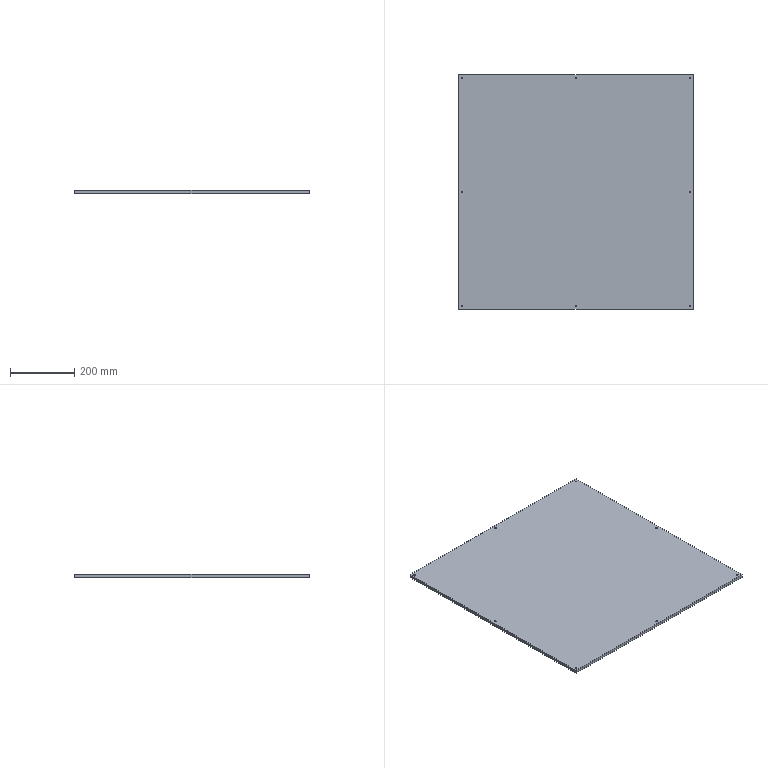Part | STEP file | SynoNew-0304-059 | 1 solid | 14 faces | box 730 x 730 x 10 mm | volume 5327429 mm3 | cylinder 8 | plane 6 | commonest cylinder face diameters 5 x8
STEP:
#1=CARTESIAN_POINT('',(-352.5,-355.,10.));
#2=VERTEX_POINT('',#1);
#3=CARTESIAN_POINT('',(-357.5,-355.,10.));
#4=VERTEX_POINT('',#3);
#5=CARTESIAN_POINT('',(-355.,-355.,10.));
#6=DIRECTION('',(0.,0.,-1.));
#7=DIRECTION('',(1.,0.,0.));
#8=AXIS2_PLACEMENT_3D('',#5,#6,#7);
#9=CIRCLE('',#8,2.5);
#10=EDGE_CURVE('',#2,#4,#9,.T.);
#11=ORIENTED_EDGE('',*,*,#10,.F.);
#12=CARTESIAN_POINT('',(-355.,-355.,10.));
#13=DIRECTION('',(0.,0.,-1.));
#14=DIRECTION('',(1.,0.,0.));
#15=AXIS2_PLACEMENT_3D('',#12,#13,#14);
#16=CIRCLE('',#15,2.5);
#17=EDGE_CURVE('',#4,#2,#16,.T.);
#18=ORIENTED_EDGE('',*,*,#17,.F.);
#19=CARTESIAN_POINT('',(-357.5,-355.,0.));
#20=VERTEX_POINT('',#19);
#21=CARTESIAN_POINT('',(-357.5,-355.,-1022.424));
#22=DIRECTION('',(0.,0.,-1.));
#23=VECTOR('',#22,2.5);
#24=LINE('',#21,#23);
#25=EDGE_CURVE('',#4,#20,#24,.T.);
#26=ORIENTED_EDGE('',*,*,#25,.T.);
#27=CARTESIAN_POINT('',(-355.,-355.,0.));
#28=DIRECTION('',(0.,0.,1.));
#29=DIRECTION('',(1.,0.,0.));
#30=AXIS2_PLACEMENT_3D('',#27,#28,#29);
#31=CIRCLE('',#30,2.5);
#32=EDGE_CURVE('',#20,#20,#31,.T.);
#33=ORIENTED_EDGE('',*,*,#32,.F.);
#34=ORIENTED_EDGE('',*,*,#25,.F.);
#35=EDGE_LOOP('',(#11,#18,#26,#33,#34));
#36=FACE_OUTER_BOUND('',#35,.T.);
#37=CARTESIAN_POINT('',(-355.,-355.,-1022.424));
#38=DIRECTION('',(0.,0.,1.));
#39=DIRECTION('',(1.,0.,0.));
#40=AXIS2_PLACEMENT_3D('',#37,#38,#39);
#41=CYLINDRICAL_SURFACE('',#40,2.5);
#42=ADVANCED_FACE('',(#36),#41,.F.);
#43=CARTESIAN_POINT('',(357.5,-355.,10.));
#44=VERTEX_POINT('',#43);
#45=CARTESIAN_POINT('',(352.5,-355.,10.));
#46=VERTEX_POINT('',#45);
#47=CARTESIAN_POINT('',(355.,-355.,10.));
#48=DIRECTION('',(0.,0.,-1.));
#49=DIRECTION('',(1.,0.,0.));
#50=AXIS2_PLACEMENT_3D('',#47,#48,#49);
#51=CIRCLE('',#50,2.5);
#52=EDGE_CURVE('',#44,#46,#51,.T.);
#53=ORIENTED_EDGE('',*,*,#52,.F.);
#54=CARTESIAN_POINT('',(355.,-355.,10.));
#55=DIRECTION('',(0.,0.,-1.));
#56=DIRECTION('',(1.,0.,0.));
#57=AXIS2_PLACEMENT_3D('',#54,#55,#56);
#58=CIRCLE('',#57,2.5);
#59=EDGE_CURVE('',#46,#44,#58,.T.);
#60=ORIENTED_EDGE('',*,*,#59,.F.);
#61=CARTESIAN_POINT('',(352.5,-355.,0.));
#62=VERTEX_POINT('',#61);
#63=CARTESIAN_POINT('',(352.5,-355.,-1022.424));
#64=DIRECTION('',(0.,0.,-1.));
#65=VECTOR('',#64,2.5);
#66=LINE('',#63,#65);
#67=EDGE_CURVE('',#46,#62,#66,.T.);
#68=ORIENTED_EDGE('',*,*,#67,.T.);
#69=CARTESIAN_POINT('',(355.,-355.,0.));
#70=DIRECTION('',(0.,0.,1.));
#71=DIRECTION('',(1.,0.,0.));
#72=AXIS2_PLACEMENT_3D('',#69,#70,#71);
#73=CIRCLE('',#72,2.5);
#74=EDGE_CURVE('',#62,#62,#73,.T.);
#75=ORIENTED_EDGE('',*,*,#74,.F.);
#76=ORIENTED_EDGE('',*,*,#67,.F.);
#77=EDGE_LOOP('',(#53,#60,#68,#75,#76));
#78=FACE_OUTER_BOUND('',#77,.T.);
#79=CARTESIAN_POINT('',(355.,-355.,-1022.424));
#80=DIRECTION('',(0.,0.,1.));
#81=DIRECTION('',(1.,0.,0.));
#82=AXIS2_PLACEMENT_3D('',#79,#80,#81);
#83=CYLINDRICAL_SURFACE('',#82,2.5);
#84=ADVANCED_FACE('',(#78),#83,.F.);
#85=CARTESIAN_POINT('',(2.5,355.,10.));
#86=VERTEX_POINT('',#85);
#87=CARTESIAN_POINT('',(-2.5,355.,10.));
#88=VERTEX_POINT('',#87);
#89=CARTESIAN_POINT('',(0.,355.,10.));
#90=DIRECTION('',(0.,0.,-1.));
#91=DIRECTION('',(1.,0.,0.));
#92=AXIS2_PLACEMENT_3D('',#89,#90,#91);
#93=CIRCLE('',#92,2.5);
#94=EDGE_CURVE('',#86,#88,#93,.T.);
#95=ORIENTED_EDGE('',*,*,#94,.F.);
#96=CARTESIAN_POINT('',(0.,355.,10.));
#97=DIRECTION('',(0.,0.,-1.));
#98=DIRECTION('',(1.,0.,0.));
#99=AXIS2_PLACEMENT_3D('',#96,#97,#98);
#100=CIRCLE('',#99,2.5);
#101=EDGE_CURVE('',#88,#86,#100,.T.);
#102=ORIENTED_EDGE('',*,*,#101,.F.);
#103=CARTESIAN_POINT('',(-2.5,355.,0.));
#104=VERTEX_POINT('',#103);
#105=CARTESIAN_POINT('',(-2.5,355.,-1022.424));
#106=DIRECTION('',(0.,0.,-1.));
#107=VECTOR('',#106,2.5);
#108=LINE('',#105,#107);
#109=EDGE_CURVE('',#88,#104,#108,.T.);
#110=ORIENTED_EDGE('',*,*,#109,.T.);
#111=CARTESIAN_POINT('',(0.,355.,0.));
#112=DIRECTION('',(0.,0.,1.));
#113=DIRECTION('',(1.,0.,0.));
#114=AXIS2_PLACEMENT_3D('',#111,#112,#113);
#115=CIRCLE('',#114,2.5);
#116=EDGE_CURVE('',#104,#104,#115,.T.);
#117=ORIENTED_EDGE('',*,*,#116,.F.);
#118=ORIENTED_EDGE('',*,*,#109,.F.);
#119=EDGE_LOOP('',(#95,#102,#110,#117,#118));
#120=FACE_OUTER_BOUND('',#119,.T.);
#121=CARTESIAN_POINT('',(0.,355.,-1022.424));
#122=DIRECTION('',(0.,0.,1.));
#123=DIRECTION('',(1.,0.,0.));
#124=AXIS2_PLACEMENT_3D('',#121,#122,#123);
#125=CYLINDRICAL_SURFACE('',#124,2.5);
#126=ADVANCED_FACE('',(#120),#125,.F.);
#127=CARTESIAN_POINT('',(-352.5,355.,10.));
#128=VERTEX_POINT('',#127);
#129=CARTESIAN_POINT('',(-357.5,355.,10.));
#130=VERTEX_POINT('',#129);
#131=CARTESIAN_POINT('',(-355.,355.,10.));
#132=DIRECTION('',(0.,0.,-1.));
#133=DIRECTION('',(1.,0.,0.));
#134=AXIS2_PLACEMENT_3D('',#131,#132,#133);
#135=CIRCLE('',#134,2.5);
#136=EDGE_CURVE('',#128,#130,#135,.T.);
#137=ORIENTED_EDGE('',*,*,#136,.F.);
#138=CARTESIAN_POINT('',(-355.,355.,10.));
#139=DIRECTION('',(0.,0.,-1.));
#140=DIRECTION('',(1.,0.,0.));
#141=AXIS2_PLACEMENT_3D('',#138,#139,#140);
#142=CIRCLE('',#141,2.5);
#143=EDGE_CURVE('',#130,#128,#142,.T.);
#144=ORIENTED_EDGE('',*,*,#143,.F.);
#145=CARTESIAN_POINT('',(-357.5,355.,0.));
#146=VERTEX_POINT('',#145);
#147=CARTESIAN_POINT('',(-357.5,355.,-1022.424));
#148=DIRECTION('',(0.,0.,-1.));
#149=VECTOR('',#148,2.5);
#150=LINE('',#147,#149);
#151=EDGE_CURVE('',#130,#146,#150,.T.);
#152=ORIENTED_EDGE('',*,*,#151,.T.);
#153=CARTESIAN_POINT('',(-355.,355.,0.));
#154=DIRECTION('',(0.,0.,1.));
#155=DIRECTION('',(1.,0.,0.));
#156=AXIS2_PLACEMENT_3D('',#153,#154,#155);
#157=CIRCLE('',#156,2.5);
#158=EDGE_CURVE('',#146,#146,#157,.T.);
#159=ORIENTED_EDGE('',*,*,#158,.F.);
#160=ORIENTED_EDGE('',*,*,#151,.F.);
#161=EDGE_LOOP('',(#137,#144,#152,#159,#160));
#162=FACE_OUTER_BOUND('',#161,.T.);
#163=CARTESIAN_POINT('',(-355.,355.,-1022.424));
#164=DIRECTION('',(0.,0.,1.));
#165=DIRECTION('',(1.,0.,0.));
#166=AXIS2_PLACEMENT_3D('',#163,#164,#165);
#167=CYLINDRICAL_SURFACE('',#166,2.5);
#168=ADVANCED_FACE('',(#162),#167,.F.);
#169=CARTESIAN_POINT('',(357.5,355.,10.));
#170=VERTEX_POINT('',#169);
#171=CARTESIAN_POINT('',(352.5,355.,10.));
#172=VERTEX_POINT('',#171);
#173=CARTESIAN_POINT('',(355.,355.,10.));
#174=DIRECTION('',(0.,0.,-1.));
#175=DIRECTION('',(1.,0.,0.));
#176=AXIS2_PLACEMENT_3D('',#173,#174,#175);
#177=CIRCLE('',#176,2.5);
#178=EDGE_CURVE('',#170,#172,#177,.T.);
#179=ORIENTED_EDGE('',*,*,#178,.F.);
#180=CARTESIAN_POINT('',(355.,355.,10.));
#181=DIRECTION('',(0.,0.,-1.));
#182=DIRECTION('',(1.,0.,0.));
#183=AXIS2_PLACEMENT_3D('',#180,#181,#182);
#184=CIRCLE('',#183,2.5);
#185=EDGE_CURVE('',#172,#170,#184,.T.);
#186=ORIENTED_EDGE('',*,*,#185,.F.);
#187=CARTESIAN_POINT('',(352.5,355.,0.));
#188=VERTEX_POINT('',#187);
#189=CARTESIAN_POINT('',(352.5,355.,-1022.424));
#190=DIRECTION('',(0.,0.,-1.));
#191=VECTOR('',#190,2.5);
#192=LINE('',#189,#191);
#193=EDGE_CURVE('',#172,#188,#192,.T.);
#194=ORIENTED_EDGE('',*,*,#193,.T.);
#195=CARTESIAN_POINT('',(355.,355.,0.));
#196=DIRECTION('',(0.,0.,1.));
#197=DIRECTION('',(1.,0.,0.));
#198=AXIS2_PLACEMENT_3D('',#195,#196,#197);
#199=CIRCLE('',#198,2.5);
#200=EDGE_CURVE('',#188,#188,#199,.T.);
#201=ORIENTED_EDGE('',*,*,#200,.F.);
#202=ORIENTED_EDGE('',*,*,#193,.F.);
#203=EDGE_LOOP('',(#179,#186,#194,#201,#202));
#204=FACE_OUTER_BOUND('',#203,.T.);
#205=CARTESIAN_POINT('',(355.,355.,-1022.424));
#206=DIRECTION('',(0.,0.,1.));
#207=DIRECTION('',(1.,0.,0.));
#208=AXIS2_PLACEMENT_3D('',#205,#206,#207);
#209=CYLINDRICAL_SURFACE('',#208,2.5);
#210=ADVANCED_FACE('',(#204),#209,.F.);
#211=CARTESIAN_POINT('',(357.5,0.,10.));
#212=VERTEX_POINT('',#211);
#213=CARTESIAN_POINT('',(352.5,0.,10.));
#214=VERTEX_POINT('',#213);
#215=CARTESIAN_POINT('',(355.,0.,10.));
#216=DIRECTION('',(0.,0.,-1.));
#217=DIRECTION('',(1.,0.,0.));
#218=AXIS2_PLACEMENT_3D('',#215,#216,#217);
#219=CIRCLE('',#218,2.5);
#220=EDGE_CURVE('',#212,#214,#219,.T.);
#221=ORIENTED_EDGE('',*,*,#220,.F.);
#222=CARTESIAN_POINT('',(355.,0.,10.));
#223=DIRECTION('',(0.,0.,-1.));
#224=DIRECTION('',(1.,0.,0.));
#225=AXIS2_PLACEMENT_3D('',#222,#223,#224);
#226=CIRCLE('',#225,2.5);
#227=EDGE_CURVE('',#214,#212,#226,.T.);
#228=ORIENTED_EDGE('',*,*,#227,.F.);
#229=CARTESIAN_POINT('',(352.5,0.,0.));
#230=VERTEX_POINT('',#229);
#231=CARTESIAN_POINT('',(352.5,0.,-1022.424));
#232=DIRECTION('',(0.,0.,-1.));
#233=VECTOR('',#232,2.5);
#234=LINE('',#231,#233);
#235=EDGE_CURVE('',#214,#230,#234,.T.);
#236=ORIENTED_EDGE('',*,*,#235,.T.);
#237=CARTESIAN_POINT('',(355.,0.,0.));
#238=DIRECTION('',(0.,0.,1.));
#239=DIRECTION('',(1.,0.,0.));
#240=AXIS2_PLACEMENT_3D('',#237,#238,#239);
#241=CIRCLE('',#240,2.5);
#242=EDGE_CURVE('',#230,#230,#241,.T.);
#243=ORIENTED_EDGE('',*,*,#242,.F.);
#244=ORIENTED_EDGE('',*,*,#235,.F.);
#245=EDGE_LOOP('',(#221,#228,#236,#243,#244));
#246=FACE_OUTER_BOUND('',#245,.T.);
#247=CARTESIAN_POINT('',(355.,0.,-1022.424));
#248=DIRECTION('',(0.,0.,1.));
#249=DIRECTION('',(1.,0.,0.));
#250=AXIS2_PLACEMENT_3D('',#247,#248,#249);
#251=CYLINDRICAL_SURFACE('',#250,2.5);
#252=ADVANCED_FACE('',(#246),#251,.F.);
#253=CARTESIAN_POINT('',(2.5,-355.,10.));
#254=VERTEX_POINT('',#253);
#255=CARTESIAN_POINT('',(-2.5,-355.,10.));
#256=VERTEX_POINT('',#255);
#257=CARTESIAN_POINT('',(0.,-355.,10.));
#258=DIRECTION('',(0.,0.,-1.));
#259=DIRECTION('',(1.,0.,0.));
#260=AXIS2_PLACEMENT_3D('',#257,#258,#259);
#261=CIRCLE('',#260,2.5);
#262=EDGE_CURVE('',#254,#256,#261,.T.);
#263=ORIENTED_EDGE('',*,*,#262,.F.);
#264=CARTESIAN_POINT('',(0.,-355.,10.));
#265=DIRECTION('',(0.,0.,-1.));
#266=DIRECTION('',(1.,0.,0.));
#267=AXIS2_PLACEMENT_3D('',#264,#265,#266);
#268=CIRCLE('',#267,2.5);
#269=EDGE_CURVE('',#256,#254,#268,.T.);
#270=ORIENTED_EDGE('',*,*,#269,.F.);
#271=CARTESIAN_POINT('',(-2.5,-355.,0.));
#272=VERTEX_POINT('',#271);
#273=CARTESIAN_POINT('',(-2.5,-355.,-1022.424));
#274=DIRECTION('',(0.,0.,-1.));
#275=VECTOR('',#274,2.5);
#276=LINE('',#273,#275);
#277=EDGE_CURVE('',#256,#272,#276,.T.);
#278=ORIENTED_EDGE('',*,*,#277,.T.);
#279=CARTESIAN_POINT('',(0.,-355.,0.));
#280=DIRECTION('',(0.,0.,1.));
#281=DIRECTION('',(1.,0.,0.));
#282=AXIS2_PLACEMENT_3D('',#279,#280,#281);
#283=CIRCLE('',#282,2.5);
#284=EDGE_CURVE('',#272,#272,#283,.T.);
#285=ORIENTED_EDGE('',*,*,#284,.F.);
#286=ORIENTED_EDGE('',*,*,#277,.F.);
#287=EDGE_LOOP('',(#263,#270,#278,#285,#286));
#288=FACE_OUTER_BOUND('',#287,.T.);
#289=CARTESIAN_POINT('',(0.,-355.,-1022.424));
#290=DIRECTION('',(0.,0.,1.));
#291=DIRECTION('',(1.,0.,0.));
#292=AXIS2_PLACEMENT_3D('',#289,#290,#291);
#293=CYLINDRICAL_SURFACE('',#292,2.5);
#294=ADVANCED_FACE('',(#288),#293,.F.);
#295=CARTESIAN_POINT('',(-352.5,0.,10.));
#296=VERTEX_POINT('',#295);
#297=CARTESIAN_POINT('',(-357.5,0.,10.));
#298=VERTEX_POINT('',#297);
#299=CARTESIAN_POINT('',(-355.,0.,10.));
#300=DIRECTION('',(0.,0.,-1.));
#301=DIRECTION('',(1.,0.,0.));
#302=AXIS2_PLACEMENT_3D('',#299,#300,#301);
#303=CIRCLE('',#302,2.5);
#304=EDGE_CURVE('',#296,#298,#303,.T.);
#305=ORIENTED_EDGE('',*,*,#304,.F.);
#306=CARTESIAN_POINT('',(-355.,0.,10.));
#307=DIRECTION('',(0.,0.,-1.));
#308=DIRECTION('',(1.,0.,0.));
#309=AXIS2_PLACEMENT_3D('',#306,#307,#308);
#310=CIRCLE('',#309,2.5);
#311=EDGE_CURVE('',#298,#296,#310,.T.);
#312=ORIENTED_EDGE('',*,*,#311,.F.);
#313=CARTESIAN_POINT('',(-357.5,0.,0.));
#314=VERTEX_POINT('',#313);
#315=CARTESIAN_POINT('',(-357.5,0.,-1022.424));
#316=DIRECTION('',(0.,0.,-1.));
#317=VECTOR('',#316,2.5);
#318=LINE('',#315,#317);
#319=EDGE_CURVE('',#298,#314,#318,.T.);
#320=ORIENTED_EDGE('',*,*,#319,.T.);
#321=CARTESIAN_POINT('',(-355.,0.,0.));
#322=DIRECTION('',(0.,0.,1.));
#323=DIRECTION('',(1.,0.,0.));
#324=AXIS2_PLACEMENT_3D('',#321,#322,#323);
#325=CIRCLE('',#324,2.5);
#326=EDGE_CURVE('',#314,#314,#325,.T.);
#327=ORIENTED_EDGE('',*,*,#326,.F.);
#328=ORIENTED_EDGE('',*,*,#319,.F.);
#329=EDGE_LOOP('',(#305,#312,#320,#327,#328));
#330=FACE_OUTER_BOUND('',#329,.T.);
#331=CARTESIAN_POINT('',(-355.,0.,-1022.424));
#332=DIRECTION('',(0.,0.,1.));
#333=DIRECTION('',(1.,0.,0.));
#334=AXIS2_PLACEMENT_3D('',#331,#332,#333);
#335=CYLINDRICAL_SURFACE('',#334,2.5);
#336=ADVANCED_FACE('',(#330),#335,.F.);
#337=CARTESIAN_POINT('',(-365.,-365.,0.));
#338=VERTEX_POINT('',#337);
#339=CARTESIAN_POINT('',(365.,-365.,0.));
#340=VERTEX_POINT('',#339);
#341=CARTESIAN_POINT('',(-365.,-365.,0.));
#342=DIRECTION('',(1.,0.,0.));
#343=VECTOR('',#342,10.);
#344=LINE('',#341,#343);
#345=EDGE_CURVE('',#338,#340,#344,.T.);
#346=ORIENTED_EDGE('',*,*,#345,.T.);
#347=CARTESIAN_POINT('',(365.,-365.,10.));
#348=VERTEX_POINT('',#347);
#349=CARTESIAN_POINT('',(365.,-365.,0.));
#350=DIRECTION('',(0.,0.,1.));
#351=VECTOR('',#350,10.);
#352=LINE('',#349,#351);
#353=EDGE_CURVE('',#340,#348,#352,.T.);
#354=ORIENTED_EDGE('',*,*,#353,.T.);
#355=CARTESIAN_POINT('',(-365.,-365.,10.));
#356=VERTEX_POINT('',#355);
#357=CARTESIAN_POINT('',(-365.,-365.,10.));
#358=DIRECTION('',(1.,0.,0.));
#359=VECTOR('',#358,10.);
#360=LINE('',#357,#359);
#361=EDGE_CURVE('',#356,#348,#360,.T.);
#362=ORIENTED_EDGE('',*,*,#361,.F.);
#363=CARTESIAN_POINT('',(-365.,-365.,0.));
#364=DIRECTION('',(0.,0.,1.));
#365=VECTOR('',#364,10.);
#366=LINE('',#363,#365);
#367=EDGE_CURVE('',#338,#356,#366,.T.);
#368=ORIENTED_EDGE('',*,*,#367,.F.);
#369=EDGE_LOOP('',(#346,#354,#362,#368));
#370=FACE_OUTER_BOUND('',#369,.T.);
#371=CARTESIAN_POINT('',(-365.,-365.,0.));
#372=DIRECTION('',(0.,-1.,0.));
#373=DIRECTION('',(1.,0.,0.));
#374=AXIS2_PLACEMENT_3D('',#371,#372,#373);
#375=PLANE('',#374);
#376=ADVANCED_FACE('',(#370),#375,.T.);
#377=CARTESIAN_POINT('',(-365.,365.,0.));
#378=VERTEX_POINT('',#377);
#379=CARTESIAN_POINT('',(-365.,365.,0.));
#380=DIRECTION('',(0.,-1.,0.));
#381=VECTOR('',#380,10.);
#382=LINE('',#379,#381);
#383=EDGE_CURVE('',#378,#338,#382,.T.);
#384=ORIENTED_EDGE('',*,*,#383,.T.);
#385=ORIENTED_EDGE('',*,*,#367,.T.);
#386=CARTESIAN_POINT('',(-365.,365.,10.));
#387=VERTEX_POINT('',#386);
#388=CARTESIAN_POINT('',(-365.,365.,10.));
#389=DIRECTION('',(0.,-1.,0.));
#390=VECTOR('',#389,10.);
#391=LINE('',#388,#390);
#392=EDGE_CURVE('',#387,#356,#391,.T.);
#393=ORIENTED_EDGE('',*,*,#392,.F.);
#394=CARTESIAN_POINT('',(-365.,365.,0.));
#395=DIRECTION('',(0.,0.,1.));
#396=VECTOR('',#395,10.);
#397=LINE('',#394,#396);
#398=EDGE_CURVE('',#378,#387,#397,.T.);
#399=ORIENTED_EDGE('',*,*,#398,.F.);
#400=EDGE_LOOP('',(#384,#385,#393,#399));
#401=FACE_OUTER_BOUND('',#400,.T.);
#402=CARTESIAN_POINT('',(-365.,365.,0.));
#403=DIRECTION('',(-1.,0.,0.));
#404=DIRECTION('',(0.,-1.,0.));
#405=AXIS2_PLACEMENT_3D('',#402,#403,#404);
#406=PLANE('',#405);
#407=ADVANCED_FACE('',(#401),#406,.T.);
#408=CARTESIAN_POINT('',(365.,365.,0.));
#409=VERTEX_POINT('',#408);
#410=CARTESIAN_POINT('',(365.,365.,0.));
#411=DIRECTION('',(-1.,0.,0.));
#412=VECTOR('',#411,10.);
#413=LINE('',#410,#412);
#414=EDGE_CURVE('',#409,#378,#413,.T.);
#415=ORIENTED_EDGE('',*,*,#414,.T.);
#416=ORIENTED_EDGE('',*,*,#398,.T.);
#417=CARTESIAN_POINT('',(365.,365.,10.));
#418=VERTEX_POINT('',#417);
#419=CARTESIAN_POINT('',(365.,365.,10.));
#420=DIRECTION('',(-1.,0.,0.));
#421=VECTOR('',#420,10.);
#422=LINE('',#419,#421);
#423=EDGE_CURVE('',#418,#387,#422,.T.);
#424=ORIENTED_EDGE('',*,*,#423,.F.);
#425=CARTESIAN_POINT('',(365.,365.,0.));
#426=DIRECTION('',(0.,0.,1.));
#427=VECTOR('',#426,10.);
#428=LINE('',#425,#427);
#429=EDGE_CURVE('',#409,#418,#428,.T.);
#430=ORIENTED_EDGE('',*,*,#429,.F.);
#431=EDGE_LOOP('',(#415,#416,#424,#430));
#432=FACE_OUTER_BOUND('',#431,.T.);
#433=CARTESIAN_POINT('',(365.,365.,0.));
#434=DIRECTION('',(0.,1.,0.));
#435=DIRECTION('',(-1.,0.,0.));
#436=AXIS2_PLACEMENT_3D('',#433,#434,#435);
#437=PLANE('',#436);
#438=ADVANCED_FACE('',(#432),#437,.T.);
#439=CARTESIAN_POINT('',(365.,-365.,0.));
#440=DIRECTION('',(0.,1.,0.));
#441=VECTOR('',#440,10.);
#442=LINE('',#439,#441);
#443=EDGE_CURVE('',#340,#409,#442,.T.);
#444=ORIENTED_EDGE('',*,*,#443,.T.);
#445=ORIENTED_EDGE('',*,*,#429,.T.);
#446=CARTESIAN_POINT('',(365.,-365.,10.));
#447=DIRECTION('',(0.,1.,0.));
#448=VECTOR('',#447,10.);
#449=LINE('',#446,#448);
#450=EDGE_CURVE('',#348,#418,#449,.T.);
#451=ORIENTED_EDGE('',*,*,#450,.F.);
#452=ORIENTED_EDGE('',*,*,#353,.F.);
#453=EDGE_LOOP('',(#444,#445,#451,#452));
#454=FACE_OUTER_BOUND('',#453,.T.);
#455=CARTESIAN_POINT('',(365.,-365.,0.));
#456=DIRECTION('',(1.,0.,0.));
#457=DIRECTION('',(0.,1.,0.));
#458=AXIS2_PLACEMENT_3D('',#455,#456,#457);
#459=PLANE('',#458);
#460=ADVANCED_FACE('',(#454),#459,.T.);
#461=ORIENTED_EDGE('',*,*,#450,.T.);
#462=ORIENTED_EDGE('',*,*,#423,.T.);
#463=ORIENTED_EDGE('',*,*,#392,.T.);
#464=ORIENTED_EDGE('',*,*,#361,.T.);
#465=EDGE_LOOP('',(#461,#462,#463,#464));
#466=FACE_OUTER_BOUND('',#465,.T.);
#467=ORIENTED_EDGE('',*,*,#10,.T.);
#468=ORIENTED_EDGE('',*,*,#17,.T.);
#469=EDGE_LOOP('',(#467,#468));
#470=FACE_BOUND('',#469,.T.);
#471=ORIENTED_EDGE('',*,*,#52,.T.);
#472=ORIENTED_EDGE('',*,*,#59,.T.);
#473=EDGE_LOOP('',(#471,#472));
#474=FACE_BOUND('',#473,.T.);
#475=ORIENTED_EDGE('',*,*,#94,.T.);
#476=ORIENTED_EDGE('',*,*,#101,.T.);
#477=EDGE_LOOP('',(#475,#476));
#478=FACE_BOUND('',#477,.T.);
#479=ORIENTED_EDGE('',*,*,#136,.T.);
#480=ORIENTED_EDGE('',*,*,#143,.T.);
#481=EDGE_LOOP('',(#479,#480));
#482=FACE_BOUND('',#481,.T.);
#483=ORIENTED_EDGE('',*,*,#178,.T.);
#484=ORIENTED_EDGE('',*,*,#185,.T.);
#485=EDGE_LOOP('',(#483,#484));
#486=FACE_BOUND('',#485,.T.);
#487=ORIENTED_EDGE('',*,*,#220,.T.);
#488=ORIENTED_EDGE('',*,*,#227,.T.);
#489=EDGE_LOOP('',(#487,#488));
#490=FACE_BOUND('',#489,.T.);
#491=ORIENTED_EDGE('',*,*,#262,.T.);
#492=ORIENTED_EDGE('',*,*,#269,.T.);
#493=EDGE_LOOP('',(#491,#492));
#494=FACE_BOUND('',#493,.T.);
#495=ORIENTED_EDGE('',*,*,#304,.T.);
#496=ORIENTED_EDGE('',*,*,#311,.T.);
#497=EDGE_LOOP('',(#495,#496));
#498=FACE_BOUND('',#497,.T.);
#499=CARTESIAN_POINT('',(0.,0.,10.));
#500=DIRECTION('',(0.,0.,1.));
#501=DIRECTION('',(1.,0.,0.));
#502=AXIS2_PLACEMENT_3D('',#499,#500,#501);
#503=PLANE('',#502);
#504=ADVANCED_FACE('',(#466,#470,#474,#478,#482,#486,#490,#494,#498),#503,.T.);
#505=ORIENTED_EDGE('',*,*,#443,.F.);
#506=ORIENTED_EDGE('',*,*,#345,.F.);
#507=ORIENTED_EDGE('',*,*,#383,.F.);
#508=ORIENTED_EDGE('',*,*,#414,.F.);
#509=EDGE_LOOP('',(#505,#506,#507,#508));
#510=FACE_OUTER_BOUND('',#509,.T.);
#511=ORIENTED_EDGE('',*,*,#32,.T.);
#512=EDGE_LOOP('',(#511));
#513=FACE_BOUND('',#512,.T.);
#514=ORIENTED_EDGE('',*,*,#74,.T.);
#515=EDGE_LOOP('',(#514));
#516=FACE_BOUND('',#515,.T.);
#517=ORIENTED_EDGE('',*,*,#116,.T.);
#518=EDGE_LOOP('',(#517));
#519=FACE_BOUND('',#518,.T.);
#520=ORIENTED_EDGE('',*,*,#158,.T.);
#521=EDGE_LOOP('',(#520));
#522=FACE_BOUND('',#521,.T.);
#523=ORIENTED_EDGE('',*,*,#200,.T.);
#524=EDGE_LOOP('',(#523));
#525=FACE_BOUND('',#524,.T.);
#526=ORIENTED_EDGE('',*,*,#242,.T.);
#527=EDGE_LOOP('',(#526));
#528=FACE_BOUND('',#527,.T.);
#529=ORIENTED_EDGE('',*,*,#284,.T.);
#530=EDGE_LOOP('',(#529));
#531=FACE_BOUND('',#530,.T.);
#532=ORIENTED_EDGE('',*,*,#326,.T.);
#533=EDGE_LOOP('',(#532));
#534=FACE_BOUND('',#533,.T.);
#535=CARTESIAN_POINT('',(0.,0.,0.));
#536=DIRECTION('',(0.,0.,1.));
#537=DIRECTION('',(1.,0.,0.));
#538=AXIS2_PLACEMENT_3D('',#535,#536,#537);
#539=PLANE('',#538);
#540=ADVANCED_FACE('',(#510,#513,#516,#519,#522,#525,#528,#531,#534),#539,.F.);
#541=CLOSED_SHELL('',(#42,#84,#126,#168,#210,#252,#294,#336,#376,#407,#438,#460,#504,#540));
#542=MANIFOLD_SOLID_BREP('',#541);
#543=(LENGTH_UNIT()NAMED_UNIT(*)SI_UNIT(.MILLI.,.METRE.));
#544=UNCERTAINTY_MEASURE_WITH_UNIT(LENGTH_MEASURE(0.01),#543,'','');
#545=(NAMED_UNIT(*)PLANE_ANGLE_UNIT()SI_UNIT($,.RADIAN.));
#546=(NAMED_UNIT(*)SI_UNIT($,.STERADIAN.)SOLID_ANGLE_UNIT());
#547=(GEOMETRIC_REPRESENTATION_CONTEXT(3)GLOBAL_UNCERTAINTY_ASSIGNED_CONTEXT((#544))GLOBAL_UNIT_ASSIGNED_CONTEXT((#543,#545,#546))REPRESENTATION_CONTEXT('',''));
#548=ADVANCED_BREP_SHAPE_REPRESENTATION('',(#542),#547);